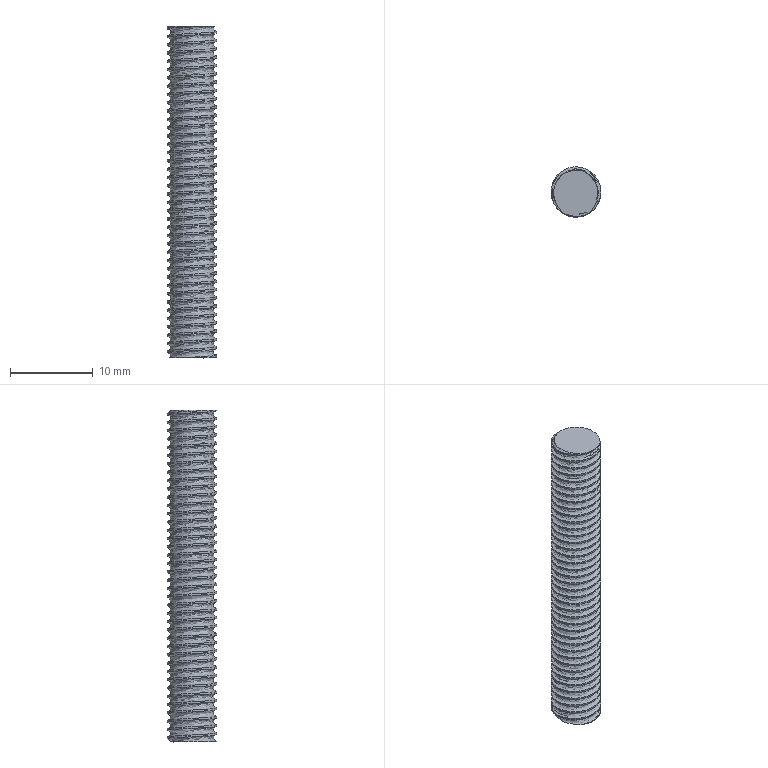Part | NX | 1 solid | 84 faces | box 6 x 6 x 40 mm | volume 952.137 mm3 | cylinder 81 | plane 2 | spline 1 | commonest cylinder face diameters 6 x81